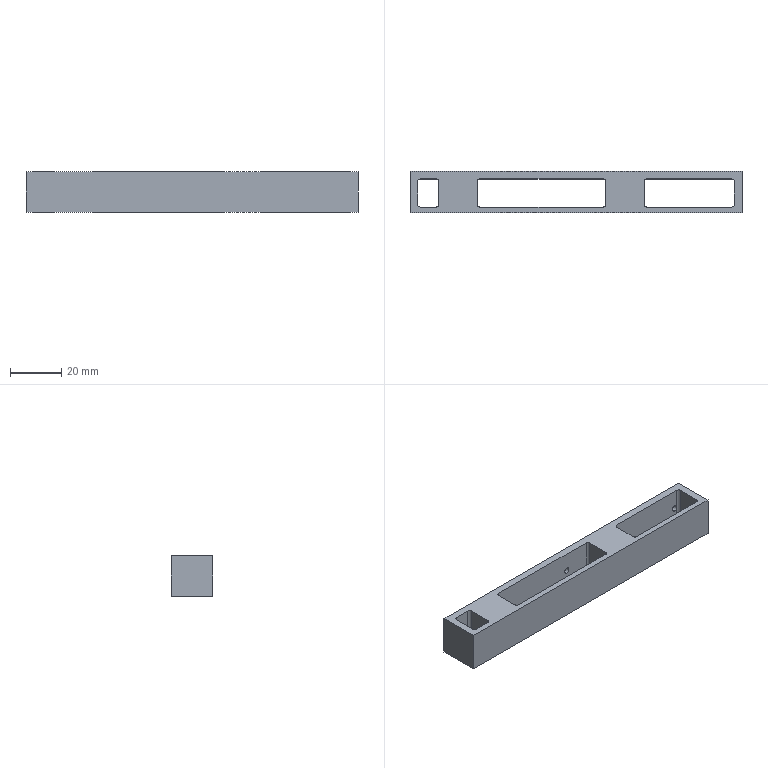NC program | NX | posted with a generic post | part box 130 x 16.2 x 16 mm
Whole program:
N10 G17 G21 G94 G90
(DRILLING , TOOL : D6A45)
N12 T07 M6
N14 G54
N16 G17 G0 G90 X-59.8 Y0. B0. C0. S5000 M3
N18 G43 Z30. H7
N20 G94 G81 G98 Z-1.6 F250. R3.
N22 X59.8
N24 X0.
N26 G80
N28 G0 X0. Y0. Z30.
N30 M5
(DRILLING_COPY , TOOL : 2.6ZT)
N32 T12 M6
N34 G54
N36 G17 G0 G90 X-59.8 Y0. B0. C0. S2000 M3
N38 G43 Z30. H12
N40 G94 G83 G98 Z-5.221 F120. Q2. R3.
N42 X59.8
N44 X0.
N46 G80
N48 G0 X0. Y0. Z30.
N50 M5
N52 M2